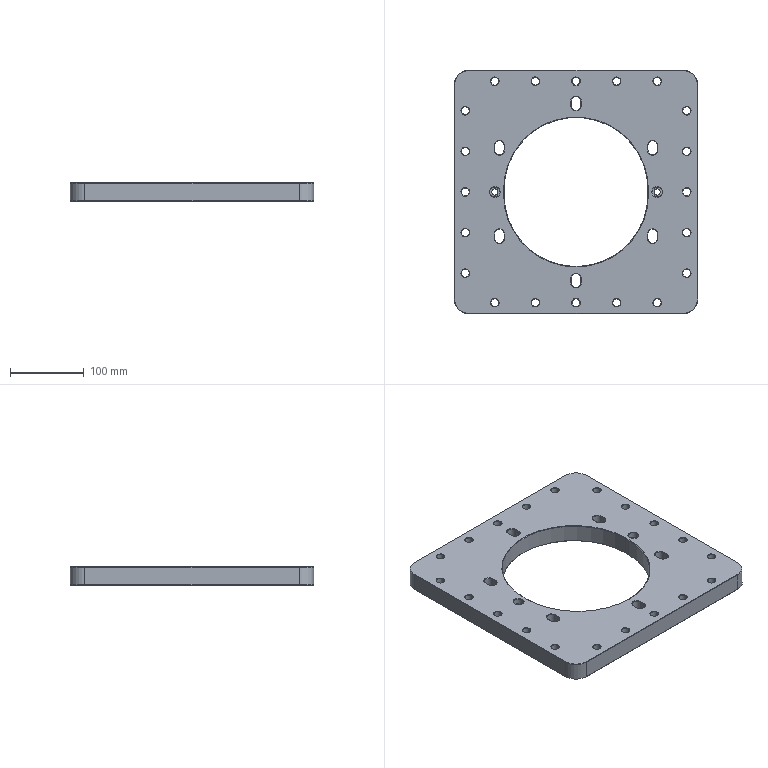Part | SolidWorks | features BaseBody 1 | 1 solid | 323 faces | box 330 x 330 x 25 mm | volume 1816926 mm3 | cone 133 | cylinder 110 | plane 80 | commonest cylinder face diameters 10.5 x40 16.5 x40 13 x12 8.5 x4 13.5 x4 16 x4